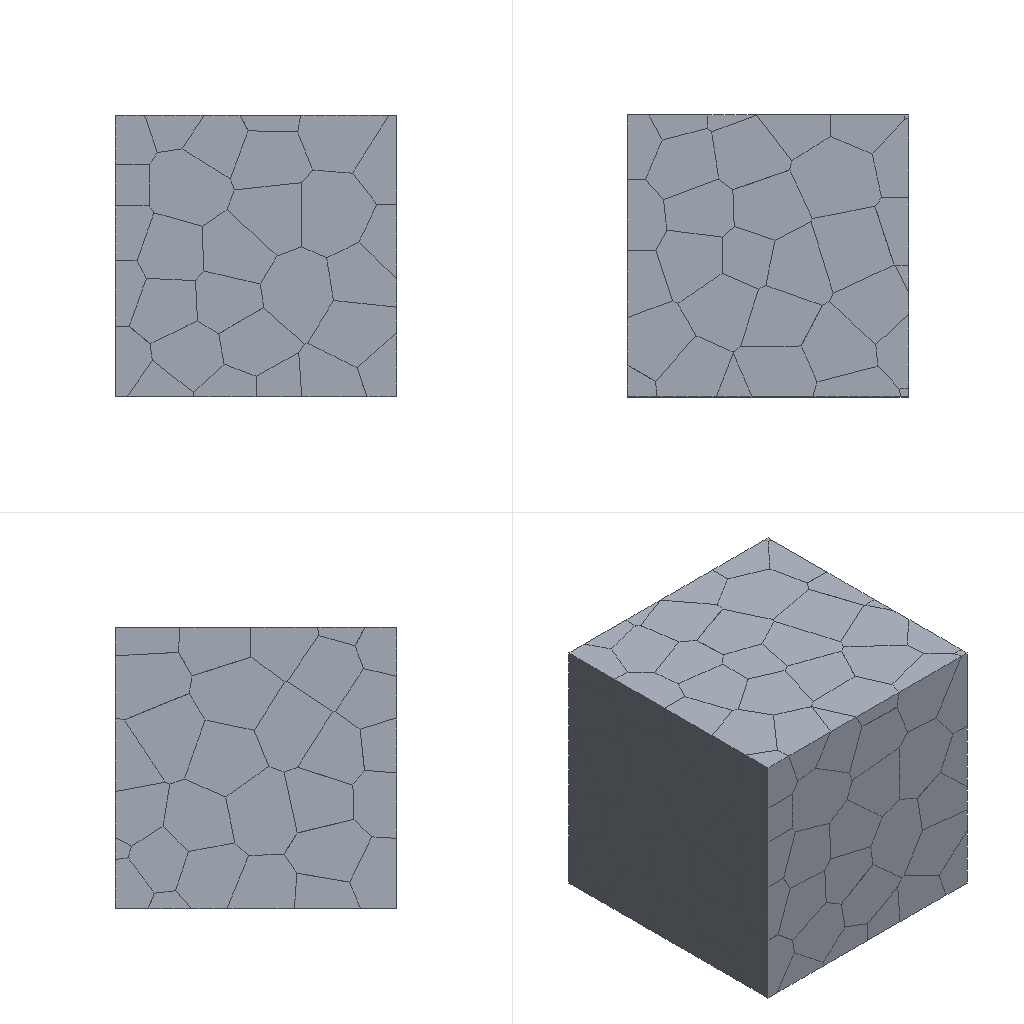Simulation study | abaqus
Set-up summary:
category,name,step,type,value,unit,region
solver,abaqus
solver,version,,,Abaqus/Standard 2020
units,not stated in the deck,,not stated
analysis,deck,,static,static
load_step,Step-1,Step-1,static,nlgeom=True
contact,interactions,,,general=0 pairs=0 ties=0
load_step,requested,,,1
mesh,nodes,,,49765
mesh,elements,,,200423
element_type,C3D4,,solid,200423
load,load commands in deck,,count,1
bc,support commands in deck,,count,3
material,DANHUAGUI,,in results
material,WUSUANKANG,,in results
check,setup vs results,,match,"per instance, exact: element labels, types and connectivity; labels of the nodes the elements use; coordinates of those nodes at SINGLE_PRECISION in 1 of 1 instance(s)"
Abaqus input file, long lists of numbers shortened:
*Heading
** Job name: Job-1 Model name: Model-1
** Generated by: Abaqus/CAE 2020
*Preprint, echo=NO, model=NO, history=NO, contact=NO
**
** PARTS
**
*Part, name=work
*Node
      1,   87.031,   39.393,   6.645
      2,   87.847,   37.972,   7.216
** (49763 more lines like these left out)
*Element, type=C3D4
  1, 30013, 30014, 30015, 30016
  2, 30017, 30018, 30014, 30019
** (200421 more lines like these left out)
*Nset, nset=Set-4
     3,     4,     9,    10,    15,    16,    17,    18,    19,    20,    21,    22,    23,    24,    25,    26
    27,    28,    29,    30,    31,    32,    33,    34,    35,    36,    37,    38,    39,    40,    41,    42
** (320 more lines like these left out)
*Elset, elset=Set-4
    601,    602,    603,    604,    605,    606,    607,    608,    609,    610,    611,    612,    613,    614,    615,    616
    617,    618,    619,    620,    621,    622,    623,    624,    625,    626,    627,    628,    629,    630,    631,    632
** (1152 more lines like these left out)
*Nset, nset=Set-5
    22,    23,    25,    26,    29,    30,    31,    32,    33,    34,    35,    36,    37,    38,    39,    40
    41,    42,    43,    44,    45,    46,    47,    49,    50,    51,    52,    53,    54,    55,    56,    57
** (425 more lines like these left out)
*Elset, elset=Set-5
   2116,   2117,   2118,   2119,   2120,   2121,   2122,   2123,   2124,   2125,   2126,   2127,   2128,   2129,   2130,   2131
   2132,   2133,   2134,   2135,   2136,   2137,   2138,   2139,   2140,   2141,   2142,   2143,   2144,   2145,   2146,   2147
** (1589 more lines like these left out)
*Nset, nset=Set-6
     1,     5,     6,    12,    13,    53,    54,    56,    57,    58,    61,    62,    64,    65,    66,    67
    68,    69,    72,    73,    76,    78,    79,    80,    83,    84,    85,    86,    87,    88,    89,   129
** (431 more lines like these left out)
*Elset, elset=Set-6
  20587,  20588,  20589,  20590,  20591,  20592,  20593,  20594,  20595,  20596,  20597,  20598,  20599,  20600,  20601,  20602
  20603,  20604,  20605,  20606,  20607,  20608,  20609,  20610,  20611,  20612,  20613,  20614,  20615,  20616,  20617,  20618
** (1687 more lines like these left out)
*Nset, nset=Set-7
     1,     2,     4,     5,     6,     7,    10,    11,    12,    60,    62,    63,    64,    65,    66,    72
    73,    74,    75,   131,   132,   133,   154,   155,   156,   157,   158,   159,   160,   161,   162,   163
** (414 more lines like these left out)
*Elset, elset=Set-7
  10321,  10322,  10323,  10324,  10325,  10326,  10327,  10328,  10329,  10330,  10331,  10332,  10333,  10334,  10335,  10336
  10337,  10338,  10339,  10340,  10341,  10342,  10343,  10344,  10345,  10346,  10347,  10348,  10349,  10350,  10351,  10352
** (1614 more lines like these left out)
*Nset, nset=Set-8
     1,     2,     3,     4,     5,     6,     7,     8,     9,    10,    11,    12,    13,    14,    16,    17
    21,    22,    23,    24,    29,    32,    39,    40,    51,    52,    53,    54,    63,    66,    71,    73
** (429 more lines like these left out)
*Elset, elset=Set-8
      1,      2,      3,      4,      5,      6,      7,      8,      9,     10,     11,     12,     13,     14,     15,     16
     17,     18,     19,     20,     21,     22,     23,     24,     25,     26,     27,     28,     29,     30,     31,     32
** (1692 more lines like these left out)
*Nset, nset=Set-9
     1,     2,     3,     4,     5,    52,    53,    55,    56,   119,   122,   123,   124,   129,   131,   132
   134,   142,   143,   145,   146,   148,   149,   150,   152,   153,   154,   155,   156,   157,   158,   159
** (423 more lines like these left out)
*Elset, elset=Set-9
   9458,   9459,   9460,   9461,   9462,   9463,   9464,   9465,   9466,   9467,   9468,   9469,   9470,   9471,   9472,   9473
   9474,   9475,   9476,   9477,   9478,   9479,   9480,   9481,   9482,   9483,   9484,   9485,   9486,   9487,   9488,   9489
** (1711 more lines like these left out)
*Nset, nset=Set-10
    17,    18,    19,    24,    27,    28,    60,    61,    62,    77,    78,    81,    82,    83,    91,    92
    94,    95,    96,   100,   101,   102,   103,   104,   105,   106,   107,   108,   109,   110,   140,   141
** (250 more lines like these left out)
*Elset, elset=Set-10
   5296,   5297,   5298,   5299,   5300,   5301,   5302,   5303,   5304,   5305,   5306,   5307,   5308,   5309,   5310,   5311
   5312,   5313,   5314,   5315,   5316,   5317,   5318,   5319,   5320,   5321,   5322,   5323,   5324,   5325,   5326,   5327
** (969 more lines like these left out)
*Nset, nset=Set-11
     2,     3,     7,     8,     9,    25,    26,    27,    28,    86,    87,    88,    90,    91,    92,    93
    96,    98,    99,   100,   101,   102,   103,   104,   105,   110,   111,   113,   114,   115,   117,   118
** (326 more lines like these left out)
*Elset, elset=Set-11
  11001,  11002,  11003,  11004,  11005,  11006,  11007,  11008,  11009,  11010,  11011,  11012,  11013,  11014,  11015,  11016
  11017,  11018,  11019,  11020,  11021,  11022,  11023,  11024,  11025,  11026,  11027,  11028,  11029,  11030,  11031,  11032
** (1329 more lines like these left out)
*Nset, nset=Set-12
    11,    12,    13,    14,    15,    16,    17,    18,    76,    77,    78,   119,   120,   121,   122,   129
   130,   131,   133,   134,   137,   138,   139,   155,   156,   159,   162,   165,   170,   185,   186,   188
** (117 more lines like these left out)
*Elset, elset=Set-12
  45499,  45500,  45501,  45502,  45503,  45504,  45505,  45506,  45507,  45508,  45509,  45510,  45511,  45512,  45513,  45514
  45515,  45516,  45517,  45518,  45519,  45520,  45521,  45522,  45523,  45524,  45525,  45526,  45527,  45528,  45529,  45530
** (442 more lines like these left out)
*Nset, nset=Set-13
    23,    24,    26,    27,   112,   113,   116,   117,   189,   190,   191,   192,   196,   197,   198,   202
   203,   204,   209,   210,   239,   240,   241,   242,   244,   247,   248,   264,   265,   266,   272,   273
** (83 more lines like these left out)
*Elset, elset=Set-13
  42876,  42877,  42878,  42879,  42880,  42881,  42882,  42883,  42884,  42885,  42886,  42887,  42888,  42889,  42890,  42891
  42892,  42893,  42894,  42895,  42896,  42897,  42898,  42899,  42900,  42901,  42902,  42903,  42904,  42905,  42906,  42907
** (324 more lines like these left out)
** Section: Section-1
*Solid Section, elset=Set-8, material=wusuankang
,
** Section: Section-1
*Solid Section, elset=Set-4, material=wusuankang
,
** Section: danhuagui
*Solid Section, elset=Set-5, material=danhuagui
,
** Section: Section-1
*Solid Section, elset=Set-10, material=wusuankang
,
** Section: danhuagui
*Solid Section, elset=Set-9, material=danhuagui
,
** Section: danhuagui
*Solid Section, elset=Set-7, material=danhuagui
,
** Section: danhuagui
*Solid Section, elset=Set-11, material=danhuagui
,
** Section: Section-1
*Solid Section, elset=Set-6, material=wusuankang
,
** Section: danhuagui
*Solid Section, elset=Set-13, material=danhuagui
,
** Section: Section-1
*Solid Section, elset=Set-12, material=wusuankang
,
*End Part
**
**
** ASSEMBLY
**
*Assembly, name=Assembly
**
*Instance, name=work-1, part=work
*End Instance
**
*Nset, nset=Set-1, instance=work-1, generate
     1,  49765,      1
*Elset, elset=Set-1, instance=work-1, generate
      1,  200423,       1
*Nset, nset=Set-2, instance=work-1
     8,     9,    10,    11,    14,    19,    20,    21,    22,    25,    26,    28,    33,    34,    35,    36
    41,    42,    45,    47,    48,    91,    94,    95,    97,   106,   107,   108,   109,   112,   116,   125
** (145 more lines like these left out)
*Elset, elset=Set-2, instance=work-1
     14,     17,     18,     19,     67,     82,    105,    112,    121,    152,    160,    177,    178,    180,    197,    214
    226,    245,    257,    258,    261,    288,    290,    296,    297,    300,    307,    315,    317,    320,    326,    328
** (266 more lines like these left out)
*Nset, nset=Set-3, instance=work-1
     6,     7,     8,    13,    14,    15,    18,    19,    20,    29,    30,    33,    35,    37,    40,    42
    43,    48,    49,    51,    54,    57,    67,    68,    69,    70,    72,    75,    81,    82,    84,    89
** (147 more lines like these left out)
*Elset, elset=Set-3, instance=work-1
     27,     67,    105,    112,    124,    157,    191,    192,    210,    250,    251,    253,    262,    286,    288,    290
    292,    307,    315,    320,    321,    324,    338,    341,    347,    351,    378,    379,    381,    382,    384,    387
** (264 more lines like these left out)
*Nset, nset=Set-4, instance=work-1
    15,    16,    20,    21,    47,    48,    49,    50,    51,    52,    55,   119,   120,   123,   126,   127
   128,   140,   141,   145,   146,   147,   173,   174,   175,   178,   184,   185,   186,   197,   198,   207
** (147 more lines like these left out)
*Elset, elset=Set-4, instance=work-1
    637,    715,    724,    812,    824,    852,    863,    919,    922,    955,    974,   1027,   1062,   1063,   1066,   1077
   1084,   1086,   1087,   1088,   1089,   1091,   1092,   1093,   1094,   1095,   1108,   1109,   1110,   1113,   1118,   1119
** (271 more lines like these left out)
*End Assembly
*Amplitude, name=Amp-1
             0.,              0.,              1.,              1.
**
** MATERIALS
**
*Material, name=danhuagui
*Density
 3.15e-09,
*Elastic
250000., 0.29
*Expansion
 2.7e-06,
*Material, name=wusuankang
*Density
 6e-09,
*Elastic
150000., 0.25
*Expansion
 -1e-06,
**
** PREDEFINED FIELDS
**
** Name: Predefined Field-1   Type: Temperature
*Initial Conditions, type=TEMPERATURE
Set-1, 1000.
** ----------------------------------------------------------------
**
** STEP: Step-1
**
*Step, name=Step-1, nlgeom=YES, inc=10000
*Static, stabilize=0.0002, allsdtol=0.05, continue=NO
0.01, 1., 1e-05, 0.1
**
** BOUNDARY CONDITIONS
**
** Name: BC-1 Type: 位移/转角
*Boundary
Set-2, 1, 1
** Name: BC-2 Type: 位移/转角
*Boundary
Set-3, 3, 3
** Name: BC-3 Type: 位移/转角
*Boundary
Set-4, 2, 2
**
** PREDEFINED FIELDS
**
** Name: Predefined Field-1   Type: Temperature
*Temperature, amplitude=Amp-1
Set-1, 20.
**
** OUTPUT REQUESTS
**
*Restart, write, number interval=1, time marks=NO
**
** FIELD OUTPUT: F-Output-1
**
*Output, field
*Node Output
CF, RF, RM, RT, U, V
*Element Output, directions=YES
E, LE, MISES, MISESMAX, MISESONLY, NE, PE, PEEQ, PEEQMAX, PEEQT, PEMAG, PRESSONLY, S, SEQUT, SSAVG, TEMP
TSHR, YIELDPOT
*Contact Output
CDISP, CSTRESS
**
** HISTORY OUTPUT: H-Output-1
**
*Output, history, variable=PRESELECT
*End Step
Results summary:
result,step,,completed,increments=16 time=1.0/1.0
result,analysis,,,static
result,last_loadstep,,,1
result,analysis steps,,count,1
result,primary field,,,U
result,reaction total,,FX,3.923,model units
result,reaction total,,FY,-4.656,model units
result,reaction total,,FZ,2.558,model units